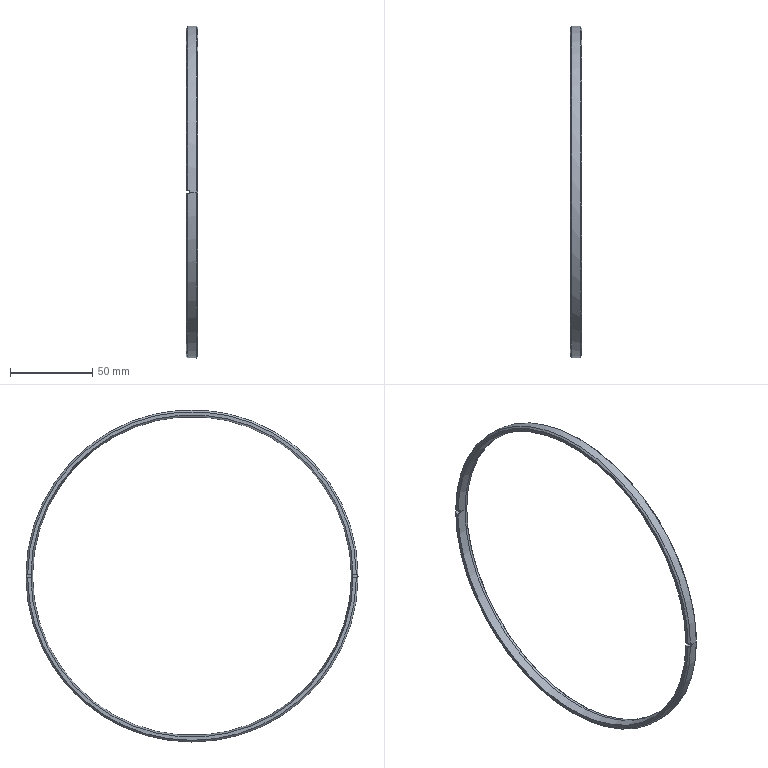Part | STEP file | pressure ring 1.stp.STEP-212.STEP | 1 solid | 22 faces | box 7 x 202 x 202 mm | volume 15156 mm3 | cone 9 | plane 9 | cylinder 4 | commonest cylinder face diameters 194 x2 202 x2
STEP:
#1=CARTESIAN_POINT('',(27.369,0.,-100.));
#2=VERTEX_POINT('',#1);
#3=CARTESIAN_POINT('',(27.369,0.,100.));
#4=VERTEX_POINT('',#3);
#5=CARTESIAN_POINT('',(27.369,0.,0.));
#6=DIRECTION('',(1.,0.,0.));
#7=DIRECTION('',(0.,0.,1.));
#8=AXIS2_PLACEMENT_3D('',#5,#6,#7);
#9=CIRCLE('',#8,100.);
#10=EDGE_CURVE('',#2,#4,#9,.T.);
#11=ORIENTED_EDGE('',*,*,#10,.F.);
#12=CARTESIAN_POINT('',(26.369,0.,-101.));
#13=VERTEX_POINT('',#12);
#14=CARTESIAN_POINT('',(26.369,0.,-101.));
#15=DIRECTION('',(-0.7071,0.,-0.7071));
#16=VECTOR('',#15,1000.);
#17=LINE('',#14,#16);
#18=EDGE_CURVE('',#2,#13,#17,.T.);
#19=ORIENTED_EDGE('',*,*,#18,.T.);
#20=CARTESIAN_POINT('',(26.369,101.,0.));
#21=VERTEX_POINT('',#20);
#22=CARTESIAN_POINT('',(26.369,0.,0.));
#23=DIRECTION('',(-1.,0.,0.));
#24=DIRECTION('',(0.,0.,1.));
#25=AXIS2_PLACEMENT_3D('',#22,#23,#24);
#26=CIRCLE('',#25,101.);
#27=EDGE_CURVE('',#21,#13,#26,.T.);
#28=ORIENTED_EDGE('',*,*,#27,.F.);
#29=CARTESIAN_POINT('',(26.369,0.,101.));
#30=VERTEX_POINT('',#29);
#31=CARTESIAN_POINT('',(26.369,0.,0.));
#32=DIRECTION('',(-1.,0.,0.));
#33=DIRECTION('',(0.,0.,1.));
#34=AXIS2_PLACEMENT_3D('',#31,#32,#33);
#35=CIRCLE('',#34,101.);
#36=EDGE_CURVE('',#30,#21,#35,.T.);
#37=ORIENTED_EDGE('',*,*,#36,.F.);
#38=CARTESIAN_POINT('',(26.369,0.,101.));
#39=DIRECTION('',(-0.7071,0.,0.7071));
#40=VECTOR('',#39,1000.);
#41=LINE('',#38,#40);
#42=EDGE_CURVE('',#4,#30,#41,.T.);
#43=ORIENTED_EDGE('',*,*,#42,.F.);
#44=EDGE_LOOP('',(#11,#19,#28,#37,#43));
#45=FACE_OUTER_BOUND('',#44,.T.);
#46=CARTESIAN_POINT('',(26.369,0.,0.));
#47=DIRECTION('',(-1.,0.,0.));
#48=DIRECTION('',(0.,0.,1.));
#49=AXIS2_PLACEMENT_3D('',#46,#47,#48);
#50=CONICAL_SURFACE('',#49,101.,0.7854);
#51=ADVANCED_FACE('',(#45),#50,.T.);
#52=CARTESIAN_POINT('',(20.369,0.,-100.));
#53=VERTEX_POINT('',#52);
#54=CARTESIAN_POINT('',(20.369,-99.995,-1.));
#55=VERTEX_POINT('',#54);
#56=CARTESIAN_POINT('',(20.369,0.,0.));
#57=DIRECTION('',(-1.,0.,0.));
#58=DIRECTION('',(0.,0.,-1.));
#59=AXIS2_PLACEMENT_3D('',#56,#57,#58);
#60=CIRCLE('',#59,100.);
#61=EDGE_CURVE('',#53,#55,#60,.T.);
#62=ORIENTED_EDGE('',*,*,#61,.F.);
#63=CARTESIAN_POINT('',(21.369,0.,-101.));
#64=VERTEX_POINT('',#63);
#65=CARTESIAN_POINT('',(20.369,0.,-100.));
#66=DIRECTION('',(0.7071,0.,-0.7071));
#67=VECTOR('',#66,1000.);
#68=LINE('',#65,#67);
#69=EDGE_CURVE('',#53,#64,#68,.T.);
#70=ORIENTED_EDGE('',*,*,#69,.T.);
#71=CARTESIAN_POINT('',(21.369,-100.995,-1.));
#72=VERTEX_POINT('',#71);
#73=CARTESIAN_POINT('',(21.369,0.,0.));
#74=DIRECTION('',(1.,0.,0.));
#75=DIRECTION('',(0.,0.,-1.));
#76=AXIS2_PLACEMENT_3D('',#73,#74,#75);
#77=CIRCLE('',#76,101.);
#78=EDGE_CURVE('',#72,#64,#77,.T.);
#79=ORIENTED_EDGE('',*,*,#78,.F.);
#80=CARTESIAN_POINT('',(20.369,-99.995,-1.));
#81=CARTESIAN_POINT('',(20.703,-100.328,-1.));
#82=CARTESIAN_POINT('',(21.036,-100.662,-1.));
#83=CARTESIAN_POINT('',(21.369,-100.995,-1.));
#84=B_SPLINE_CURVE_WITH_KNOTS('',3,(#80,#81,#82,#83),.UNSPECIFIED.,.F.,.F.,(4,4),(0.,0.001414),.UNSPECIFIED.);
#85=EDGE_CURVE('',#55,#72,#84,.T.);
#86=ORIENTED_EDGE('',*,*,#85,.F.);
#87=EDGE_LOOP('',(#62,#70,#79,#86));
#88=FACE_OUTER_BOUND('',#87,.T.);
#89=CARTESIAN_POINT('',(20.369,0.,0.));
#90=DIRECTION('',(1.,0.,0.));
#91=DIRECTION('',(0.,0.,-1.));
#92=AXIS2_PLACEMENT_3D('',#89,#90,#91);
#93=CONICAL_SURFACE('',#92,100.,0.7854);
#94=ADVANCED_FACE('',(#88),#93,.T.);
#95=CARTESIAN_POINT('',(25.369,-97.,0.));
#96=VERTEX_POINT('',#95);
#97=CARTESIAN_POINT('',(25.369,97.,0.));
#98=VERTEX_POINT('',#97);
#99=CARTESIAN_POINT('',(25.369,0.,0.));
#100=DIRECTION('',(-1.,0.,0.));
#101=DIRECTION('',(0.,1.,0.));
#102=AXIS2_PLACEMENT_3D('',#99,#100,#101);
#103=CIRCLE('',#102,97.);
#104=EDGE_CURVE('',#96,#98,#103,.T.);
#105=ORIENTED_EDGE('',*,*,#104,.F.);
#106=CARTESIAN_POINT('',(22.369,-97.6,0.));
#107=VERTEX_POINT('',#106);
#108=CARTESIAN_POINT('',(20.369,-98.,0.));
#109=DIRECTION('',(-0.9806,-0.1961,0.));
#110=VECTOR('',#109,1000.);
#111=LINE('',#108,#110);
#112=EDGE_CURVE('',#96,#107,#111,.T.);
#113=ORIENTED_EDGE('',*,*,#112,.T.);
#114=CARTESIAN_POINT('',(22.369,-97.595,1.));
#115=VERTEX_POINT('',#114);
#116=CARTESIAN_POINT('',(22.369,0.,0.));
#117=DIRECTION('',(-1.,0.,0.));
#118=DIRECTION('',(0.,0.,-1.));
#119=AXIS2_PLACEMENT_3D('',#116,#117,#118);
#120=CIRCLE('',#119,97.6);
#121=EDGE_CURVE('',#107,#115,#120,.T.);
#122=ORIENTED_EDGE('',*,*,#121,.T.);
#123=CARTESIAN_POINT('',(20.369,-97.995,1.));
#124=VERTEX_POINT('',#123);
#125=CARTESIAN_POINT('',(20.369,-97.995,1.));
#126=CARTESIAN_POINT('',(21.036,-97.862,1.));
#127=CARTESIAN_POINT('',(21.703,-97.728,1.));
#128=CARTESIAN_POINT('',(22.369,-97.595,1.));
#129=B_SPLINE_CURVE_WITH_KNOTS('',3,(#125,#126,#127,#128),.UNSPECIFIED.,.F.,.F.,(4,4),(0.1999,0.2019),.UNSPECIFIED.);
#130=EDGE_CURVE('',#124,#115,#129,.T.);
#131=ORIENTED_EDGE('',*,*,#130,.F.);
#132=CARTESIAN_POINT('',(20.369,97.995,1.));
#133=VERTEX_POINT('',#132);
#134=CARTESIAN_POINT('',(20.369,0.,0.));
#135=DIRECTION('',(-1.,0.,0.));
#136=DIRECTION('',(0.,1.,0.));
#137=AXIS2_PLACEMENT_3D('',#134,#135,#136);
#138=CIRCLE('',#137,98.);
#139=EDGE_CURVE('',#124,#133,#138,.T.);
#140=ORIENTED_EDGE('',*,*,#139,.T.);
#141=CARTESIAN_POINT('',(22.369,97.595,1.));
#142=VERTEX_POINT('',#141);
#143=CARTESIAN_POINT('',(22.369,97.595,1.));
#144=CARTESIAN_POINT('',(21.703,97.728,1.));
#145=CARTESIAN_POINT('',(21.036,97.862,1.));
#146=CARTESIAN_POINT('',(20.369,97.995,1.));
#147=B_SPLINE_CURVE_WITH_KNOTS('',3,(#143,#144,#145,#146),.UNSPECIFIED.,.F.,.F.,(4,4),(0.1999,0.2019),.UNSPECIFIED.);
#148=EDGE_CURVE('',#142,#133,#147,.T.);
#149=ORIENTED_EDGE('',*,*,#148,.F.);
#150=CARTESIAN_POINT('',(22.369,97.6,0.));
#151=VERTEX_POINT('',#150);
#152=CARTESIAN_POINT('',(22.369,0.,0.));
#153=DIRECTION('',(-1.,0.,0.));
#154=DIRECTION('',(0.,0.,-1.));
#155=AXIS2_PLACEMENT_3D('',#152,#153,#154);
#156=CIRCLE('',#155,97.6);
#157=EDGE_CURVE('',#142,#151,#156,.T.);
#158=ORIENTED_EDGE('',*,*,#157,.T.);
#159=CARTESIAN_POINT('',(20.369,98.,0.));
#160=DIRECTION('',(-0.9806,0.1961,0.));
#161=VECTOR('',#160,1000.);
#162=LINE('',#159,#161);
#163=EDGE_CURVE('',#98,#151,#162,.T.);
#164=ORIENTED_EDGE('',*,*,#163,.F.);
#165=EDGE_LOOP('',(#105,#113,#122,#131,#140,#149,#158,#164));
#166=FACE_OUTER_BOUND('',#165,.T.);
#167=CARTESIAN_POINT('',(20.369,0.,0.));
#168=DIRECTION('',(-1.,0.,0.));
#169=DIRECTION('',(0.,1.,0.));
#170=AXIS2_PLACEMENT_3D('',#167,#168,#169);
#171=CONICAL_SURFACE('',#170,98.,0.1974);
#172=ADVANCED_FACE('',(#166),#171,.F.);
#173=ORIENTED_EDGE('',*,*,#27,.T.);
#174=CARTESIAN_POINT('',(26.369,-101.,0.));
#175=VERTEX_POINT('',#174);
#176=CARTESIAN_POINT('',(26.369,0.,0.));
#177=DIRECTION('',(-1.,0.,0.));
#178=DIRECTION('',(0.,0.,1.));
#179=AXIS2_PLACEMENT_3D('',#176,#177,#178);
#180=CIRCLE('',#179,101.);
#181=EDGE_CURVE('',#13,#175,#180,.T.);
#182=ORIENTED_EDGE('',*,*,#181,.T.);
#183=CARTESIAN_POINT('',(22.369,-101.,0.));
#184=VERTEX_POINT('',#183);
#185=CARTESIAN_POINT('',(0.,-101.,0.));
#186=DIRECTION('',(-1.,0.,0.));
#187=VECTOR('',#186,1000.);
#188=LINE('',#185,#187);
#189=EDGE_CURVE('',#175,#184,#188,.T.);
#190=ORIENTED_EDGE('',*,*,#189,.T.);
#191=CARTESIAN_POINT('',(22.369,-100.995,-1.));
#192=VERTEX_POINT('',#191);
#193=CARTESIAN_POINT('',(22.369,0.,0.));
#194=DIRECTION('',(1.,0.,0.));
#195=DIRECTION('',(0.,0.,-1.));
#196=AXIS2_PLACEMENT_3D('',#193,#194,#195);
#197=CIRCLE('',#196,101.);
#198=EDGE_CURVE('',#184,#192,#197,.T.);
#199=ORIENTED_EDGE('',*,*,#198,.T.);
#200=CARTESIAN_POINT('',(0.,-100.995,-1.));
#201=DIRECTION('',(1.,0.,0.));
#202=VECTOR('',#201,1000.);
#203=LINE('',#200,#202);
#204=EDGE_CURVE('',#72,#192,#203,.T.);
#205=ORIENTED_EDGE('',*,*,#204,.F.);
#206=ORIENTED_EDGE('',*,*,#78,.T.);
#207=CARTESIAN_POINT('',(21.369,100.995,-1.));
#208=VERTEX_POINT('',#207);
#209=CARTESIAN_POINT('',(21.369,0.,0.));
#210=DIRECTION('',(1.,0.,0.));
#211=DIRECTION('',(0.,0.,-1.));
#212=AXIS2_PLACEMENT_3D('',#209,#210,#211);
#213=CIRCLE('',#212,101.);
#214=EDGE_CURVE('',#64,#208,#213,.T.);
#215=ORIENTED_EDGE('',*,*,#214,.T.);
#216=CARTESIAN_POINT('',(22.369,100.995,-1.));
#217=VERTEX_POINT('',#216);
#218=CARTESIAN_POINT('',(0.,100.995,-1.));
#219=DIRECTION('',(-1.,0.,0.));
#220=VECTOR('',#219,1000.);
#221=LINE('',#218,#220);
#222=EDGE_CURVE('',#217,#208,#221,.T.);
#223=ORIENTED_EDGE('',*,*,#222,.F.);
#224=CARTESIAN_POINT('',(22.369,101.,0.));
#225=VERTEX_POINT('',#224);
#226=CARTESIAN_POINT('',(22.369,0.,0.));
#227=DIRECTION('',(1.,0.,0.));
#228=DIRECTION('',(0.,0.,-1.));
#229=AXIS2_PLACEMENT_3D('',#226,#227,#228);
#230=CIRCLE('',#229,101.);
#231=EDGE_CURVE('',#217,#225,#230,.T.);
#232=ORIENTED_EDGE('',*,*,#231,.T.);
#233=CARTESIAN_POINT('',(0.,101.,0.));
#234=DIRECTION('',(-1.,0.,0.));
#235=VECTOR('',#234,1000.);
#236=LINE('',#233,#235);
#237=EDGE_CURVE('',#21,#225,#236,.T.);
#238=ORIENTED_EDGE('',*,*,#237,.F.);
#239=EDGE_LOOP('',(#173,#182,#190,#199,#205,#206,#215,#223,#232,#238));
#240=FACE_OUTER_BOUND('',#239,.T.);
#241=CARTESIAN_POINT('',(0.,0.,0.));
#242=DIRECTION('',(-1.,0.,0.));
#243=DIRECTION('',(0.,1.,0.));
#244=AXIS2_PLACEMENT_3D('',#241,#242,#243);
#245=CYLINDRICAL_SURFACE('',#244,101.);
#246=ADVANCED_FACE('',(#240),#245,.T.);
#247=CARTESIAN_POINT('',(26.869,-97.,0.));
#248=VERTEX_POINT('',#247);
#249=CARTESIAN_POINT('',(26.869,97.,0.));
#250=VERTEX_POINT('',#249);
#251=CARTESIAN_POINT('',(26.869,0.,0.));
#252=DIRECTION('',(-1.,0.,0.));
#253=DIRECTION('',(0.,1.,0.));
#254=AXIS2_PLACEMENT_3D('',#251,#252,#253);
#255=CIRCLE('',#254,97.);
#256=EDGE_CURVE('',#248,#250,#255,.T.);
#257=ORIENTED_EDGE('',*,*,#256,.F.);
#258=CARTESIAN_POINT('',(0.,-97.,0.));
#259=DIRECTION('',(-1.,0.,0.));
#260=VECTOR('',#259,1000.);
#261=LINE('',#258,#260);
#262=EDGE_CURVE('',#248,#96,#261,.T.);
#263=ORIENTED_EDGE('',*,*,#262,.T.);
#264=ORIENTED_EDGE('',*,*,#104,.T.);
#265=CARTESIAN_POINT('',(0.,97.,0.));
#266=DIRECTION('',(-1.,0.,0.));
#267=VECTOR('',#266,1000.);
#268=LINE('',#265,#267);
#269=EDGE_CURVE('',#250,#98,#268,.T.);
#270=ORIENTED_EDGE('',*,*,#269,.F.);
#271=EDGE_LOOP('',(#257,#263,#264,#270));
#272=FACE_OUTER_BOUND('',#271,.T.);
#273=CARTESIAN_POINT('',(0.,0.,0.));
#274=DIRECTION('',(-1.,0.,0.));
#275=DIRECTION('',(0.,1.,0.));
#276=AXIS2_PLACEMENT_3D('',#273,#274,#275);
#277=CYLINDRICAL_SURFACE('',#276,97.);
#278=ADVANCED_FACE('',(#272),#277,.F.);
#279=ORIENTED_EDGE('',*,*,#256,.T.);
#280=CARTESIAN_POINT('',(27.369,97.5,0.));
#281=VERTEX_POINT('',#280);
#282=CARTESIAN_POINT('',(26.869,97.,0.));
#283=DIRECTION('',(0.7071,0.7071,0.));
#284=VECTOR('',#283,1000.);
#285=LINE('',#282,#284);
#286=EDGE_CURVE('',#250,#281,#285,.T.);
#287=ORIENTED_EDGE('',*,*,#286,.T.);
#288=CARTESIAN_POINT('',(27.369,-97.5,0.));
#289=VERTEX_POINT('',#288);
#290=CARTESIAN_POINT('',(27.369,0.,0.));
#291=DIRECTION('',(-1.,0.,0.));
#292=DIRECTION('',(0.,1.,0.));
#293=AXIS2_PLACEMENT_3D('',#290,#291,#292);
#294=CIRCLE('',#293,97.5);
#295=EDGE_CURVE('',#289,#281,#294,.T.);
#296=ORIENTED_EDGE('',*,*,#295,.F.);
#297=CARTESIAN_POINT('',(26.869,-97.,0.));
#298=DIRECTION('',(0.7071,-0.7071,0.));
#299=VECTOR('',#298,1000.);
#300=LINE('',#297,#299);
#301=EDGE_CURVE('',#248,#289,#300,.T.);
#302=ORIENTED_EDGE('',*,*,#301,.F.);
#303=EDGE_LOOP('',(#279,#287,#296,#302));
#304=FACE_OUTER_BOUND('',#303,.T.);
#305=CARTESIAN_POINT('',(26.869,0.,0.));
#306=DIRECTION('',(1.,0.,0.));
#307=DIRECTION('',(0.,-1.,0.));
#308=AXIS2_PLACEMENT_3D('',#305,#306,#307);
#309=CONICAL_SURFACE('',#308,97.,0.7854);
#310=ADVANCED_FACE('',(#304),#309,.F.);
#311=CARTESIAN_POINT('',(20.369,99.995,-1.));
#312=VERTEX_POINT('',#311);
#313=CARTESIAN_POINT('',(20.369,97.995,-1.));
#314=VERTEX_POINT('',#313);
#315=CARTESIAN_POINT('',(20.369,110.,-1.));
#316=DIRECTION('',(0.,-1.,0.));
#317=VECTOR('',#316,1000.);
#318=LINE('',#315,#317);
#319=EDGE_CURVE('',#312,#314,#318,.T.);
#320=ORIENTED_EDGE('',*,*,#319,.F.);
#321=CARTESIAN_POINT('',(20.369,0.,0.));
#322=DIRECTION('',(-1.,0.,0.));
#323=DIRECTION('',(0.,0.,-1.));
#324=AXIS2_PLACEMENT_3D('',#321,#322,#323);
#325=CIRCLE('',#324,100.);
#326=EDGE_CURVE('',#312,#53,#325,.T.);
#327=ORIENTED_EDGE('',*,*,#326,.T.);
#328=ORIENTED_EDGE('',*,*,#61,.T.);
#329=CARTESIAN_POINT('',(20.369,-97.995,-1.));
#330=VERTEX_POINT('',#329);
#331=CARTESIAN_POINT('',(20.369,110.,-1.));
#332=DIRECTION('',(0.,-1.,0.));
#333=VECTOR('',#332,1000.);
#334=LINE('',#331,#333);
#335=EDGE_CURVE('',#330,#55,#334,.T.);
#336=ORIENTED_EDGE('',*,*,#335,.F.);
#337=CARTESIAN_POINT('',(20.369,0.,0.));
#338=DIRECTION('',(-1.,0.,0.));
#339=DIRECTION('',(0.,1.,0.));
#340=AXIS2_PLACEMENT_3D('',#337,#338,#339);
#341=CIRCLE('',#340,98.);
#342=EDGE_CURVE('',#314,#330,#341,.T.);
#343=ORIENTED_EDGE('',*,*,#342,.F.);
#344=EDGE_LOOP('',(#320,#327,#328,#336,#343));
#345=FACE_OUTER_BOUND('',#344,.T.);
#346=CARTESIAN_POINT('',(20.369,101.,0.));
#347=DIRECTION('',(1.,0.,0.));
#348=DIRECTION('',(0.,1.,0.));
#349=AXIS2_PLACEMENT_3D('',#346,#347,#348);
#350=PLANE('',#349);
#351=ADVANCED_FACE('',(#345),#350,.F.);
#352=CARTESIAN_POINT('',(22.369,-100.995,1.));
#353=VERTEX_POINT('',#352);
#354=CARTESIAN_POINT('',(21.369,-100.995,1.));
#355=VERTEX_POINT('',#354);
#356=CARTESIAN_POINT('',(0.,-100.995,1.));
#357=DIRECTION('',(-1.,0.,0.));
#358=VECTOR('',#357,1000.);
#359=LINE('',#356,#358);
#360=EDGE_CURVE('',#353,#355,#359,.T.);
#361=ORIENTED_EDGE('',*,*,#360,.T.);
#362=CARTESIAN_POINT('',(20.369,-99.995,1.));
#363=VERTEX_POINT('',#362);
#364=CARTESIAN_POINT('',(21.369,-100.995,1.));
#365=CARTESIAN_POINT('',(21.036,-100.662,1.));
#366=CARTESIAN_POINT('',(20.703,-100.328,1.));
#367=CARTESIAN_POINT('',(20.369,-99.995,1.));
#368=B_SPLINE_CURVE_WITH_KNOTS('',3,(#364,#365,#366,#367),.UNSPECIFIED.,.F.,.F.,(4,4),(0.,0.001414),.UNSPECIFIED.);
#369=EDGE_CURVE('',#355,#363,#368,.T.);
#370=ORIENTED_EDGE('',*,*,#369,.T.);
#371=CARTESIAN_POINT('',(20.369,-110.,1.));
#372=DIRECTION('',(0.,1.,0.));
#373=VECTOR('',#372,1000.);
#374=LINE('',#371,#373);
#375=EDGE_CURVE('',#363,#124,#374,.T.);
#376=ORIENTED_EDGE('',*,*,#375,.T.);
#377=ORIENTED_EDGE('',*,*,#130,.T.);
#378=CARTESIAN_POINT('',(22.369,-110.,1.));
#379=DIRECTION('',(0.,1.,0.));
#380=VECTOR('',#379,1000.);
#381=LINE('',#378,#380);
#382=EDGE_CURVE('',#353,#115,#381,.T.);
#383=ORIENTED_EDGE('',*,*,#382,.F.);
#384=EDGE_LOOP('',(#361,#370,#376,#377,#383));
#385=FACE_OUTER_BOUND('',#384,.T.);
#386=CARTESIAN_POINT('',(22.369,-110.,1.));
#387=DIRECTION('',(0.,0.,-1.));
#388=DIRECTION('',(0.,-1.,0.));
#389=AXIS2_PLACEMENT_3D('',#386,#387,#388);
#390=PLANE('',#389);
#391=ADVANCED_FACE('',(#385),#390,.T.);
#392=CARTESIAN_POINT('',(22.369,100.995,1.));
#393=VERTEX_POINT('',#392);
#394=CARTESIAN_POINT('',(22.369,-110.,1.));
#395=DIRECTION('',(0.,1.,0.));
#396=VECTOR('',#395,1000.);
#397=LINE('',#394,#396);
#398=EDGE_CURVE('',#142,#393,#397,.T.);
#399=ORIENTED_EDGE('',*,*,#398,.T.);
#400=CARTESIAN_POINT('',(22.369,0.,0.));
#401=DIRECTION('',(1.,0.,0.));
#402=DIRECTION('',(0.,0.,-1.));
#403=AXIS2_PLACEMENT_3D('',#400,#401,#402);
#404=CIRCLE('',#403,101.);
#405=EDGE_CURVE('',#225,#393,#404,.T.);
#406=ORIENTED_EDGE('',*,*,#405,.F.);
#407=ORIENTED_EDGE('',*,*,#231,.F.);
#408=CARTESIAN_POINT('',(22.369,97.595,-1.));
#409=VERTEX_POINT('',#408);
#410=CARTESIAN_POINT('',(22.369,110.,-1.));
#411=DIRECTION('',(0.,-1.,0.));
#412=VECTOR('',#411,1000.);
#413=LINE('',#410,#412);
#414=EDGE_CURVE('',#217,#409,#413,.T.);
#415=ORIENTED_EDGE('',*,*,#414,.T.);
#416=CARTESIAN_POINT('',(22.369,0.,0.));
#417=DIRECTION('',(-1.,0.,0.));
#418=DIRECTION('',(0.,0.,-1.));
#419=AXIS2_PLACEMENT_3D('',#416,#417,#418);
#420=CIRCLE('',#419,97.6);
#421=EDGE_CURVE('',#151,#409,#420,.T.);
#422=ORIENTED_EDGE('',*,*,#421,.F.);
#423=ORIENTED_EDGE('',*,*,#157,.F.);
#424=EDGE_LOOP('',(#399,#406,#407,#415,#422,#423));
#425=FACE_OUTER_BOUND('',#424,.T.);
#426=CARTESIAN_POINT('',(22.369,-25.,-25.));
#427=DIRECTION('',(1.,0.,0.));
#428=DIRECTION('',(0.,1.,0.));
#429=AXIS2_PLACEMENT_3D('',#426,#427,#428);
#430=PLANE('',#429);
#431=ADVANCED_FACE('',(#425),#430,.F.);
#432=CARTESIAN_POINT('',(20.369,99.995,1.));
#433=VERTEX_POINT('',#432);
#434=CARTESIAN_POINT('',(20.369,-110.,1.));
#435=DIRECTION('',(0.,1.,0.));
#436=VECTOR('',#435,1000.);
#437=LINE('',#434,#436);
#438=EDGE_CURVE('',#133,#433,#437,.T.);
#439=ORIENTED_EDGE('',*,*,#438,.T.);
#440=CARTESIAN_POINT('',(21.369,100.995,1.));
#441=VERTEX_POINT('',#440);
#442=CARTESIAN_POINT('',(20.369,99.995,1.));
#443=CARTESIAN_POINT('',(20.703,100.328,1.));
#444=CARTESIAN_POINT('',(21.036,100.662,1.));
#445=CARTESIAN_POINT('',(21.369,100.995,1.));
#446=B_SPLINE_CURVE_WITH_KNOTS('',3,(#442,#443,#444,#445),.UNSPECIFIED.,.F.,.F.,(4,4),(0.,0.001414),.UNSPECIFIED.);
#447=EDGE_CURVE('',#433,#441,#446,.T.);
#448=ORIENTED_EDGE('',*,*,#447,.T.);
#449=CARTESIAN_POINT('',(0.,100.995,1.));
#450=DIRECTION('',(1.,0.,0.));
#451=VECTOR('',#450,1000.);
#452=LINE('',#449,#451);
#453=EDGE_CURVE('',#441,#393,#452,.T.);
#454=ORIENTED_EDGE('',*,*,#453,.T.);
#455=ORIENTED_EDGE('',*,*,#398,.F.);
#456=ORIENTED_EDGE('',*,*,#148,.T.);
#457=EDGE_LOOP('',(#439,#448,#454,#455,#456));
#458=FACE_OUTER_BOUND('',#457,.T.);
#459=CARTESIAN_POINT('',(22.369,-110.,1.));
#460=DIRECTION('',(0.,0.,-1.));
#461=DIRECTION('',(0.,-1.,0.));
#462=AXIS2_PLACEMENT_3D('',#459,#460,#461);
#463=PLANE('',#462);
#464=ADVANCED_FACE('',(#458),#463,.T.);
#465=ORIENTED_EDGE('',*,*,#222,.T.);
#466=CARTESIAN_POINT('',(21.369,100.995,-1.));
#467=CARTESIAN_POINT('',(21.036,100.662,-1.));
#468=CARTESIAN_POINT('',(20.703,100.328,-1.));
#469=CARTESIAN_POINT('',(20.369,99.995,-1.));
#470=B_SPLINE_CURVE_WITH_KNOTS('',3,(#466,#467,#468,#469),.UNSPECIFIED.,.F.,.F.,(4,4),(0.,0.001414),.UNSPECIFIED.);
#471=EDGE_CURVE('',#208,#312,#470,.T.);
#472=ORIENTED_EDGE('',*,*,#471,.T.);
#473=ORIENTED_EDGE('',*,*,#319,.T.);
#474=CARTESIAN_POINT('',(20.369,97.995,-1.));
#475=CARTESIAN_POINT('',(21.036,97.862,-1.));
#476=CARTESIAN_POINT('',(21.703,97.728,-1.));
#477=CARTESIAN_POINT('',(22.369,97.595,-1.));
#478=B_SPLINE_CURVE_WITH_KNOTS('',3,(#474,#475,#476,#477),.UNSPECIFIED.,.F.,.F.,(4,4),(0.1999,0.2019),.UNSPECIFIED.);
#479=EDGE_CURVE('',#314,#409,#478,.T.);
#480=ORIENTED_EDGE('',*,*,#479,.T.);
#481=ORIENTED_EDGE('',*,*,#414,.F.);
#482=EDGE_LOOP('',(#465,#472,#473,#480,#481));
#483=FACE_OUTER_BOUND('',#482,.T.);
#484=CARTESIAN_POINT('',(22.369,110.,-1.));
#485=DIRECTION('',(0.,0.,1.));
#486=DIRECTION('',(0.,-1.,0.));
#487=AXIS2_PLACEMENT_3D('',#484,#485,#486);
#488=PLANE('',#487);
#489=ADVANCED_FACE('',(#483),#488,.T.);
#490=CARTESIAN_POINT('',(22.369,-97.595,-1.));
#491=VERTEX_POINT('',#490);
#492=CARTESIAN_POINT('',(22.369,110.,-1.));
#493=DIRECTION('',(0.,-1.,0.));
#494=VECTOR('',#493,1000.);
#495=LINE('',#492,#494);
#496=EDGE_CURVE('',#491,#192,#495,.T.);
#497=ORIENTED_EDGE('',*,*,#496,.T.);
#498=ORIENTED_EDGE('',*,*,#198,.F.);
#499=CARTESIAN_POINT('',(22.369,0.,0.));
#500=DIRECTION('',(1.,0.,0.));
#501=DIRECTION('',(0.,0.,-1.));
#502=AXIS2_PLACEMENT_3D('',#499,#500,#501);
#503=CIRCLE('',#502,101.);
#504=EDGE_CURVE('',#353,#184,#503,.T.);
#505=ORIENTED_EDGE('',*,*,#504,.F.);
#506=ORIENTED_EDGE('',*,*,#382,.T.);
#507=ORIENTED_EDGE('',*,*,#121,.F.);
#508=CARTESIAN_POINT('',(22.369,0.,0.));
#509=DIRECTION('',(-1.,0.,0.));
#510=DIRECTION('',(0.,0.,-1.));
#511=AXIS2_PLACEMENT_3D('',#508,#509,#510);
#512=CIRCLE('',#511,97.6);
#513=EDGE_CURVE('',#491,#107,#512,.T.);
#514=ORIENTED_EDGE('',*,*,#513,.F.);
#515=EDGE_LOOP('',(#497,#498,#505,#506,#507,#514));
#516=FACE_OUTER_BOUND('',#515,.T.);
#517=CARTESIAN_POINT('',(22.369,-25.,-25.));
#518=DIRECTION('',(1.,0.,0.));
#519=DIRECTION('',(0.,1.,0.));
#520=AXIS2_PLACEMENT_3D('',#517,#518,#519);
#521=PLANE('',#520);
#522=ADVANCED_FACE('',(#516),#521,.F.);
#523=ORIENTED_EDGE('',*,*,#295,.T.);
#524=CARTESIAN_POINT('',(27.369,0.,0.));
#525=DIRECTION('',(-1.,0.,0.));
#526=DIRECTION('',(0.,1.,0.));
#527=AXIS2_PLACEMENT_3D('',#524,#525,#526);
#528=CIRCLE('',#527,97.5);
#529=EDGE_CURVE('',#281,#289,#528,.T.);
#530=ORIENTED_EDGE('',*,*,#529,.T.);
#531=EDGE_LOOP('',(#523,#530));
#532=FACE_BOUND('',#531,.T.);
#533=CARTESIAN_POINT('',(27.369,0.,0.));
#534=DIRECTION('',(1.,0.,0.));
#535=DIRECTION('',(0.,0.,1.));
#536=AXIS2_PLACEMENT_3D('',#533,#534,#535);
#537=CIRCLE('',#536,100.);
#538=EDGE_CURVE('',#4,#2,#537,.T.);
#539=ORIENTED_EDGE('',*,*,#538,.T.);
#540=ORIENTED_EDGE('',*,*,#10,.T.);
#541=EDGE_LOOP('',(#539,#540));
#542=FACE_OUTER_BOUND('',#541,.T.);
#543=CARTESIAN_POINT('',(27.369,97.5,0.));
#544=DIRECTION('',(-1.,0.,0.));
#545=DIRECTION('',(0.,0.,1.));
#546=AXIS2_PLACEMENT_3D('',#543,#544,#545);
#547=PLANE('',#546);
#548=ADVANCED_FACE('',(#532,#542),#547,.F.);
#549=ORIENTED_EDGE('',*,*,#375,.F.);
#550=CARTESIAN_POINT('',(20.369,0.,0.));
#551=DIRECTION('',(-1.,0.,0.));
#552=DIRECTION('',(0.,0.,-1.));
#553=AXIS2_PLACEMENT_3D('',#550,#551,#552);
#554=CIRCLE('',#553,100.);
#555=EDGE_CURVE('',#363,#433,#554,.T.);
#556=ORIENTED_EDGE('',*,*,#555,.T.);
#557=ORIENTED_EDGE('',*,*,#438,.F.);
#558=ORIENTED_EDGE('',*,*,#139,.F.);
#559=EDGE_LOOP('',(#549,#556,#557,#558));
#560=FACE_OUTER_BOUND('',#559,.T.);
#561=CARTESIAN_POINT('',(20.369,101.,0.));
#562=DIRECTION('',(1.,0.,0.));
#563=DIRECTION('',(0.,1.,0.));
#564=AXIS2_PLACEMENT_3D('',#561,#562,#563);
#565=PLANE('',#564);
#566=ADVANCED_FACE('',(#560),#565,.F.);
#567=ORIENTED_EDGE('',*,*,#286,.F.);
#568=CARTESIAN_POINT('',(26.869,0.,0.));
#569=DIRECTION('',(-1.,0.,0.));
#570=DIRECTION('',(0.,1.,0.));
#571=AXIS2_PLACEMENT_3D('',#568,#569,#570);
#572=CIRCLE('',#571,97.);
#573=EDGE_CURVE('',#250,#248,#572,.T.);
#574=ORIENTED_EDGE('',*,*,#573,.T.);
#575=ORIENTED_EDGE('',*,*,#301,.T.);
#576=ORIENTED_EDGE('',*,*,#529,.F.);
#577=EDGE_LOOP('',(#567,#574,#575,#576));
#578=FACE_OUTER_BOUND('',#577,.T.);
#579=CARTESIAN_POINT('',(26.869,0.,0.));
#580=DIRECTION('',(1.,0.,0.));
#581=DIRECTION('',(0.,-1.,0.));
#582=AXIS2_PLACEMENT_3D('',#579,#580,#581);
#583=CONICAL_SURFACE('',#582,97.,0.7854);
#584=ADVANCED_FACE('',(#578),#583,.F.);
#585=ORIENTED_EDGE('',*,*,#262,.F.);
#586=ORIENTED_EDGE('',*,*,#573,.F.);
#587=ORIENTED_EDGE('',*,*,#269,.T.);
#588=CARTESIAN_POINT('',(25.369,0.,0.));
#589=DIRECTION('',(-1.,0.,0.));
#590=DIRECTION('',(0.,1.,0.));
#591=AXIS2_PLACEMENT_3D('',#588,#589,#590);
#592=CIRCLE('',#591,97.);
#593=EDGE_CURVE('',#98,#96,#592,.T.);
#594=ORIENTED_EDGE('',*,*,#593,.T.);
#595=EDGE_LOOP('',(#585,#586,#587,#594));
#596=FACE_OUTER_BOUND('',#595,.T.);
#597=CARTESIAN_POINT('',(0.,0.,0.));
#598=DIRECTION('',(-1.,0.,0.));
#599=DIRECTION('',(0.,1.,0.));
#600=AXIS2_PLACEMENT_3D('',#597,#598,#599);
#601=CYLINDRICAL_SURFACE('',#600,97.);
#602=ADVANCED_FACE('',(#596),#601,.F.);
#603=ORIENTED_EDGE('',*,*,#189,.F.);
#604=CARTESIAN_POINT('',(26.369,0.,0.));
#605=DIRECTION('',(-1.,0.,0.));
#606=DIRECTION('',(0.,0.,1.));
#607=AXIS2_PLACEMENT_3D('',#604,#605,#606);
#608=CIRCLE('',#607,101.);
#609=EDGE_CURVE('',#175,#30,#608,.T.);
#610=ORIENTED_EDGE('',*,*,#609,.T.);
#611=ORIENTED_EDGE('',*,*,#36,.T.);
#612=ORIENTED_EDGE('',*,*,#237,.T.);
#613=ORIENTED_EDGE('',*,*,#405,.T.);
#614=ORIENTED_EDGE('',*,*,#453,.F.);
#615=CARTESIAN_POINT('',(21.369,0.,0.));
#616=DIRECTION('',(1.,0.,0.));
#617=DIRECTION('',(0.,0.,-1.));
#618=AXIS2_PLACEMENT_3D('',#615,#616,#617);
#619=CIRCLE('',#618,101.);
#620=EDGE_CURVE('',#441,#355,#619,.T.);
#621=ORIENTED_EDGE('',*,*,#620,.T.);
#622=ORIENTED_EDGE('',*,*,#360,.F.);
#623=ORIENTED_EDGE('',*,*,#504,.T.);
#624=EDGE_LOOP('',(#603,#610,#611,#612,#613,#614,#621,#622,#623));
#625=FACE_OUTER_BOUND('',#624,.T.);
#626=CARTESIAN_POINT('',(0.,0.,0.));
#627=DIRECTION('',(-1.,0.,0.));
#628=DIRECTION('',(0.,1.,0.));
#629=AXIS2_PLACEMENT_3D('',#626,#627,#628);
#630=CYLINDRICAL_SURFACE('',#629,101.);
#631=ADVANCED_FACE('',(#625),#630,.T.);
#632=ORIENTED_EDGE('',*,*,#112,.F.);
#633=ORIENTED_EDGE('',*,*,#593,.F.);
#634=ORIENTED_EDGE('',*,*,#163,.T.);
#635=ORIENTED_EDGE('',*,*,#421,.T.);
#636=ORIENTED_EDGE('',*,*,#479,.F.);
#637=ORIENTED_EDGE('',*,*,#342,.T.);
#638=CARTESIAN_POINT('',(22.369,-97.595,-1.));
#639=CARTESIAN_POINT('',(21.703,-97.728,-1.));
#640=CARTESIAN_POINT('',(21.036,-97.862,-1.));
#641=CARTESIAN_POINT('',(20.369,-97.995,-1.));
#642=B_SPLINE_CURVE_WITH_KNOTS('',3,(#638,#639,#640,#641),.UNSPECIFIED.,.F.,.F.,(4,4),(0.1999,0.2019),.UNSPECIFIED.);
#643=EDGE_CURVE('',#491,#330,#642,.T.);
#644=ORIENTED_EDGE('',*,*,#643,.F.);
#645=ORIENTED_EDGE('',*,*,#513,.T.);
#646=EDGE_LOOP('',(#632,#633,#634,#635,#636,#637,#644,#645));
#647=FACE_OUTER_BOUND('',#646,.T.);
#648=CARTESIAN_POINT('',(20.369,0.,0.));
#649=DIRECTION('',(-1.,0.,0.));
#650=DIRECTION('',(0.,1.,0.));
#651=AXIS2_PLACEMENT_3D('',#648,#649,#650);
#652=CONICAL_SURFACE('',#651,98.,0.1974);
#653=ADVANCED_FACE('',(#647),#652,.F.);
#654=ORIENTED_EDGE('',*,*,#69,.F.);
#655=ORIENTED_EDGE('',*,*,#326,.F.);
#656=ORIENTED_EDGE('',*,*,#471,.F.);
#657=ORIENTED_EDGE('',*,*,#214,.F.);
#658=EDGE_LOOP('',(#654,#655,#656,#657));
#659=FACE_OUTER_BOUND('',#658,.T.);
#660=CARTESIAN_POINT('',(20.369,0.,0.));
#661=DIRECTION('',(1.,0.,0.));
#662=DIRECTION('',(0.,0.,-1.));
#663=AXIS2_PLACEMENT_3D('',#660,#661,#662);
#664=CONICAL_SURFACE('',#663,100.,0.7854);
#665=ADVANCED_FACE('',(#659),#664,.T.);
#666=ORIENTED_EDGE('',*,*,#18,.F.);
#667=ORIENTED_EDGE('',*,*,#538,.F.);
#668=ORIENTED_EDGE('',*,*,#42,.T.);
#669=ORIENTED_EDGE('',*,*,#609,.F.);
#670=ORIENTED_EDGE('',*,*,#181,.F.);
#671=EDGE_LOOP('',(#666,#667,#668,#669,#670));
#672=FACE_OUTER_BOUND('',#671,.T.);
#673=CARTESIAN_POINT('',(26.369,0.,0.));
#674=DIRECTION('',(-1.,0.,0.));
#675=DIRECTION('',(0.,0.,1.));
#676=AXIS2_PLACEMENT_3D('',#673,#674,#675);
#677=CONICAL_SURFACE('',#676,101.,0.7854);
#678=ADVANCED_FACE('',(#672),#677,.T.);
#679=ORIENTED_EDGE('',*,*,#335,.T.);
#680=ORIENTED_EDGE('',*,*,#85,.T.);
#681=ORIENTED_EDGE('',*,*,#204,.T.);
#682=ORIENTED_EDGE('',*,*,#496,.F.);
#683=ORIENTED_EDGE('',*,*,#643,.T.);
#684=EDGE_LOOP('',(#679,#680,#681,#682,#683));
#685=FACE_OUTER_BOUND('',#684,.T.);
#686=CARTESIAN_POINT('',(22.369,110.,-1.));
#687=DIRECTION('',(0.,0.,1.));
#688=DIRECTION('',(0.,-1.,0.));
#689=AXIS2_PLACEMENT_3D('',#686,#687,#688);
#690=PLANE('',#689);
#691=ADVANCED_FACE('',(#685),#690,.T.);
#692=ORIENTED_EDGE('',*,*,#369,.F.);
#693=ORIENTED_EDGE('',*,*,#620,.F.);
#694=ORIENTED_EDGE('',*,*,#447,.F.);
#695=ORIENTED_EDGE('',*,*,#555,.F.);
#696=EDGE_LOOP('',(#692,#693,#694,#695));
#697=FACE_OUTER_BOUND('',#696,.T.);
#698=CARTESIAN_POINT('',(20.369,0.,0.));
#699=DIRECTION('',(1.,0.,0.));
#700=DIRECTION('',(0.,0.,-1.));
#701=AXIS2_PLACEMENT_3D('',#698,#699,#700);
#702=CONICAL_SURFACE('',#701,100.,0.7854);
#703=ADVANCED_FACE('',(#697),#702,.T.);
#704=CLOSED_SHELL('',(#51,#94,#172,#246,#278,#310,#351,#391,#431,#464,#489,#522,#548,#566,#584,#602,#631,#653,#665,#678,#691,#703));
#705=MANIFOLD_SOLID_BREP('',#704);
#706=CARTESIAN_POINT('',(0.,0.,0.));
#707=DIRECTION('',(0.,0.,1.));
#708=DIRECTION('',(1.,0.,0.));
#709=AXIS2_PLACEMENT_3D('',#706,#707,#708);
#710=(LENGTH_UNIT()NAMED_UNIT(*)SI_UNIT(.MILLI.,.METRE.));
#711=UNCERTAINTY_MEASURE_WITH_UNIT(LENGTH_MEASURE(0.00001),#710,'','');
#712=(NAMED_UNIT(*)PLANE_ANGLE_UNIT()SI_UNIT($,.RADIAN.));
#713=(NAMED_UNIT(*)SI_UNIT($,.STERADIAN.)SOLID_ANGLE_UNIT());
#714=(GEOMETRIC_REPRESENTATION_CONTEXT(3)GLOBAL_UNCERTAINTY_ASSIGNED_CONTEXT((#711))GLOBAL_UNIT_ASSIGNED_CONTEXT((#710,#712,#713))REPRESENTATION_CONTEXT('',''));
#715=ADVANCED_BREP_SHAPE_REPRESENTATION('',(#705,#709),#714);